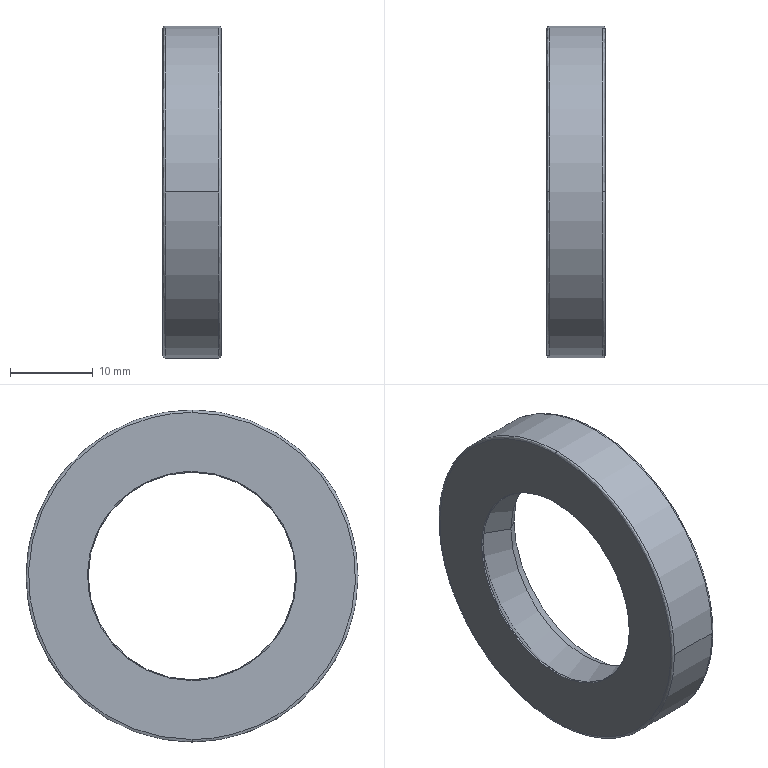Part | SolidWorks | features BaseBody 1 | 1 solid | 30 faces | box 7 x 40 x 40 mm | volume 2987 mm3 | spline 12 | cone 8 | cylinder 6 | plane 4 | commonest cylinder face diameters 29.2 x2 36.5 x2 40 x2